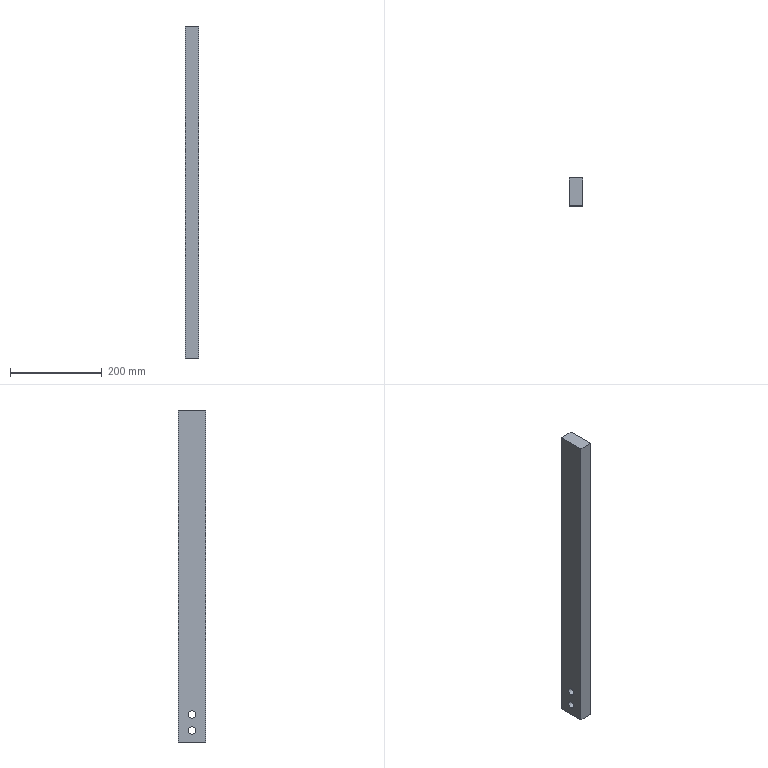Part | SolidWorks | features Cut 1, Extrusion 1, ICE 1 | 1 solid | 10 faces | box 30 x 60 x 725 mm | volume 1292936 mm3 | plane 6 | cylinder 4 | commonest cylinder face diameters 16 x4
STEP:
#1=CARTESIAN_POINT('',(15.,0.,-66.));
#2=VERTEX_POINT('',#1);
#3=CARTESIAN_POINT('',(15.,0.,-50.));
#4=VERTEX_POINT('',#3);
#5=CARTESIAN_POINT('',(15.,0.,-58.));
#6=DIRECTION('',(-1.,0.,0.));
#7=DIRECTION('',(0.,0.,1.));
#8=AXIS2_PLACEMENT_3D('',#5,#6,#7);
#9=CIRCLE('',#8,8.);
#10=EDGE_CURVE('',#2,#4,#9,.T.);
#11=ORIENTED_EDGE('',*,*,#10,.F.);
#12=CARTESIAN_POINT('',(-15.,0.,-66.));
#13=VERTEX_POINT('',#12);
#14=CARTESIAN_POINT('',(15.,0.,-66.));
#15=DIRECTION('',(-1.,0.,0.));
#16=VECTOR('',#15,1000.);
#17=LINE('',#14,#16);
#18=EDGE_CURVE('',#2,#13,#17,.T.);
#19=ORIENTED_EDGE('',*,*,#18,.T.);
#20=CARTESIAN_POINT('',(-15.,0.,-50.));
#21=VERTEX_POINT('',#20);
#22=CARTESIAN_POINT('',(-15.,0.,-58.));
#23=DIRECTION('',(-1.,0.,0.));
#24=DIRECTION('',(0.,0.,1.));
#25=AXIS2_PLACEMENT_3D('',#22,#23,#24);
#26=CIRCLE('',#25,8.);
#27=EDGE_CURVE('',#13,#21,#26,.T.);
#28=ORIENTED_EDGE('',*,*,#27,.T.);
#29=CARTESIAN_POINT('',(15.,0.,-50.));
#30=DIRECTION('',(-1.,0.,0.));
#31=VECTOR('',#30,1000.);
#32=LINE('',#29,#31);
#33=EDGE_CURVE('',#4,#21,#32,.T.);
#34=ORIENTED_EDGE('',*,*,#33,.F.);
#35=EDGE_LOOP('',(#11,#19,#28,#34));
#36=FACE_OUTER_BOUND('',#35,.T.);
#37=CARTESIAN_POINT('',(15.,0.,-58.));
#38=DIRECTION('',(-1.,0.,0.));
#39=DIRECTION('',(0.,0.,1.));
#40=AXIS2_PLACEMENT_3D('',#37,#38,#39);
#41=CYLINDRICAL_SURFACE('',#40,8.);
#42=ADVANCED_FACE('',(#36),#41,.F.);
#43=CARTESIAN_POINT('',(15.,0.,-31.));
#44=VERTEX_POINT('',#43);
#45=CARTESIAN_POINT('',(15.,0.,-15.));
#46=VERTEX_POINT('',#45);
#47=CARTESIAN_POINT('',(15.,0.,-23.));
#48=DIRECTION('',(-1.,0.,0.));
#49=DIRECTION('',(0.,0.,1.));
#50=AXIS2_PLACEMENT_3D('',#47,#48,#49);
#51=CIRCLE('',#50,8.);
#52=EDGE_CURVE('',#44,#46,#51,.T.);
#53=ORIENTED_EDGE('',*,*,#52,.F.);
#54=CARTESIAN_POINT('',(-15.,0.,-31.));
#55=VERTEX_POINT('',#54);
#56=CARTESIAN_POINT('',(15.,0.,-31.));
#57=DIRECTION('',(-1.,0.,0.));
#58=VECTOR('',#57,1000.);
#59=LINE('',#56,#58);
#60=EDGE_CURVE('',#44,#55,#59,.T.);
#61=ORIENTED_EDGE('',*,*,#60,.T.);
#62=CARTESIAN_POINT('',(-15.,0.,-15.));
#63=VERTEX_POINT('',#62);
#64=CARTESIAN_POINT('',(-15.,0.,-23.));
#65=DIRECTION('',(-1.,0.,0.));
#66=DIRECTION('',(0.,0.,1.));
#67=AXIS2_PLACEMENT_3D('',#64,#65,#66);
#68=CIRCLE('',#67,8.);
#69=EDGE_CURVE('',#55,#63,#68,.T.);
#70=ORIENTED_EDGE('',*,*,#69,.T.);
#71=CARTESIAN_POINT('',(15.,0.,-15.));
#72=DIRECTION('',(-1.,0.,0.));
#73=VECTOR('',#72,1000.);
#74=LINE('',#71,#73);
#75=EDGE_CURVE('',#46,#63,#74,.T.);
#76=ORIENTED_EDGE('',*,*,#75,.F.);
#77=EDGE_LOOP('',(#53,#61,#70,#76));
#78=FACE_OUTER_BOUND('',#77,.T.);
#79=CARTESIAN_POINT('',(15.,0.,-23.));
#80=DIRECTION('',(-1.,0.,0.));
#81=DIRECTION('',(0.,0.,1.));
#82=AXIS2_PLACEMENT_3D('',#79,#80,#81);
#83=CYLINDRICAL_SURFACE('',#82,8.);
#84=ADVANCED_FACE('',(#78),#83,.F.);
#85=CARTESIAN_POINT('',(15.,0.,-58.));
#86=DIRECTION('',(-1.,0.,0.));
#87=DIRECTION('',(0.,0.,1.));
#88=AXIS2_PLACEMENT_3D('',#85,#86,#87);
#89=CIRCLE('',#88,8.);
#90=EDGE_CURVE('',#4,#2,#89,.T.);
#91=ORIENTED_EDGE('',*,*,#90,.T.);
#92=ORIENTED_EDGE('',*,*,#10,.T.);
#93=EDGE_LOOP('',(#91,#92));
#94=FACE_BOUND('',#93,.T.);
#95=CARTESIAN_POINT('',(15.,0.,-23.));
#96=DIRECTION('',(-1.,0.,0.));
#97=DIRECTION('',(0.,0.,1.));
#98=AXIS2_PLACEMENT_3D('',#95,#96,#97);
#99=CIRCLE('',#98,8.);
#100=EDGE_CURVE('',#46,#44,#99,.T.);
#101=ORIENTED_EDGE('',*,*,#100,.T.);
#102=ORIENTED_EDGE('',*,*,#52,.T.);
#103=EDGE_LOOP('',(#101,#102));
#104=FACE_BOUND('',#103,.T.);
#105=CARTESIAN_POINT('',(15.,-30.,642.));
#106=VERTEX_POINT('',#105);
#107=CARTESIAN_POINT('',(15.,-30.,-83.));
#108=VERTEX_POINT('',#107);
#109=CARTESIAN_POINT('',(15.,-30.,642.));
#110=DIRECTION('',(0.,0.,-1.));
#111=VECTOR('',#110,1000.);
#112=LINE('',#109,#111);
#113=EDGE_CURVE('',#106,#108,#112,.T.);
#114=ORIENTED_EDGE('',*,*,#113,.T.);
#115=CARTESIAN_POINT('',(15.,30.,-83.));
#116=VERTEX_POINT('',#115);
#117=CARTESIAN_POINT('',(15.,30.,-83.));
#118=DIRECTION('',(0.,-1.,0.));
#119=VECTOR('',#118,1000.);
#120=LINE('',#117,#119);
#121=EDGE_CURVE('',#116,#108,#120,.T.);
#122=ORIENTED_EDGE('',*,*,#121,.F.);
#123=CARTESIAN_POINT('',(15.,30.,642.));
#124=VERTEX_POINT('',#123);
#125=CARTESIAN_POINT('',(15.,30.,642.));
#126=DIRECTION('',(0.,0.,-1.));
#127=VECTOR('',#126,1000.);
#128=LINE('',#125,#127);
#129=EDGE_CURVE('',#124,#116,#128,.T.);
#130=ORIENTED_EDGE('',*,*,#129,.F.);
#131=CARTESIAN_POINT('',(15.,-30.,642.));
#132=DIRECTION('',(0.,1.,0.));
#133=VECTOR('',#132,1000.);
#134=LINE('',#131,#133);
#135=EDGE_CURVE('',#106,#124,#134,.T.);
#136=ORIENTED_EDGE('',*,*,#135,.F.);
#137=EDGE_LOOP('',(#114,#122,#130,#136));
#138=FACE_OUTER_BOUND('',#137,.T.);
#139=CARTESIAN_POINT('',(15.,-30.,642.));
#140=DIRECTION('',(-1.,0.,0.));
#141=DIRECTION('',(0.,0.,1.));
#142=AXIS2_PLACEMENT_3D('',#139,#140,#141);
#143=PLANE('',#142);
#144=ADVANCED_FACE('',(#94,#104,#138),#143,.F.);
#145=ORIENTED_EDGE('',*,*,#129,.T.);
#146=CARTESIAN_POINT('',(-15.,30.,-83.));
#147=VERTEX_POINT('',#146);
#148=CARTESIAN_POINT('',(-15.,30.,-83.));
#149=DIRECTION('',(1.,0.,0.));
#150=VECTOR('',#149,1000.);
#151=LINE('',#148,#150);
#152=EDGE_CURVE('',#147,#116,#151,.T.);
#153=ORIENTED_EDGE('',*,*,#152,.F.);
#154=CARTESIAN_POINT('',(-15.,30.,642.));
#155=VERTEX_POINT('',#154);
#156=CARTESIAN_POINT('',(-15.,30.,642.));
#157=DIRECTION('',(0.,0.,-1.));
#158=VECTOR('',#157,1000.);
#159=LINE('',#156,#158);
#160=EDGE_CURVE('',#155,#147,#159,.T.);
#161=ORIENTED_EDGE('',*,*,#160,.F.);
#162=CARTESIAN_POINT('',(-15.,30.,642.));
#163=DIRECTION('',(-1.,0.,0.));
#164=VECTOR('',#163,1000.);
#165=LINE('',#162,#164);
#166=EDGE_CURVE('',#124,#155,#165,.T.);
#167=ORIENTED_EDGE('',*,*,#166,.F.);
#168=EDGE_LOOP('',(#145,#153,#161,#167));
#169=FACE_OUTER_BOUND('',#168,.T.);
#170=CARTESIAN_POINT('',(-15.,30.,642.));
#171=DIRECTION('',(0.,-1.,0.));
#172=DIRECTION('',(0.,0.,-1.));
#173=AXIS2_PLACEMENT_3D('',#170,#171,#172);
#174=PLANE('',#173);
#175=ADVANCED_FACE('',(#169),#174,.F.);
#176=CARTESIAN_POINT('',(-15.,0.,-58.));
#177=DIRECTION('',(-1.,0.,0.));
#178=DIRECTION('',(0.,0.,1.));
#179=AXIS2_PLACEMENT_3D('',#176,#177,#178);
#180=CIRCLE('',#179,8.);
#181=EDGE_CURVE('',#21,#13,#180,.T.);
#182=ORIENTED_EDGE('',*,*,#181,.F.);
#183=ORIENTED_EDGE('',*,*,#27,.F.);
#184=EDGE_LOOP('',(#182,#183));
#185=FACE_BOUND('',#184,.T.);
#186=CARTESIAN_POINT('',(-15.,0.,-23.));
#187=DIRECTION('',(-1.,0.,0.));
#188=DIRECTION('',(0.,0.,1.));
#189=AXIS2_PLACEMENT_3D('',#186,#187,#188);
#190=CIRCLE('',#189,8.);
#191=EDGE_CURVE('',#63,#55,#190,.T.);
#192=ORIENTED_EDGE('',*,*,#191,.F.);
#193=ORIENTED_EDGE('',*,*,#69,.F.);
#194=EDGE_LOOP('',(#192,#193));
#195=FACE_BOUND('',#194,.T.);
#196=ORIENTED_EDGE('',*,*,#160,.T.);
#197=CARTESIAN_POINT('',(-15.,-30.,-83.));
#198=VERTEX_POINT('',#197);
#199=CARTESIAN_POINT('',(-15.,-30.,-83.));
#200=DIRECTION('',(0.,1.,0.));
#201=VECTOR('',#200,1000.);
#202=LINE('',#199,#201);
#203=EDGE_CURVE('',#198,#147,#202,.T.);
#204=ORIENTED_EDGE('',*,*,#203,.F.);
#205=CARTESIAN_POINT('',(-15.,-30.,642.));
#206=VERTEX_POINT('',#205);
#207=CARTESIAN_POINT('',(-15.,-30.,642.));
#208=DIRECTION('',(0.,0.,-1.));
#209=VECTOR('',#208,1000.);
#210=LINE('',#207,#209);
#211=EDGE_CURVE('',#206,#198,#210,.T.);
#212=ORIENTED_EDGE('',*,*,#211,.F.);
#213=CARTESIAN_POINT('',(-15.,-30.,642.));
#214=DIRECTION('',(0.,-1.,0.));
#215=VECTOR('',#214,1000.);
#216=LINE('',#213,#215);
#217=EDGE_CURVE('',#155,#206,#216,.T.);
#218=ORIENTED_EDGE('',*,*,#217,.F.);
#219=EDGE_LOOP('',(#196,#204,#212,#218));
#220=FACE_OUTER_BOUND('',#219,.T.);
#221=CARTESIAN_POINT('',(-15.,-30.,642.));
#222=DIRECTION('',(1.,0.,0.));
#223=DIRECTION('',(0.,0.,-1.));
#224=AXIS2_PLACEMENT_3D('',#221,#222,#223);
#225=PLANE('',#224);
#226=ADVANCED_FACE('',(#185,#195,#220),#225,.F.);
#227=ORIENTED_EDGE('',*,*,#211,.T.);
#228=CARTESIAN_POINT('',(15.,-30.,-83.));
#229=DIRECTION('',(-1.,0.,0.));
#230=VECTOR('',#229,1000.);
#231=LINE('',#228,#230);
#232=EDGE_CURVE('',#108,#198,#231,.T.);
#233=ORIENTED_EDGE('',*,*,#232,.F.);
#234=ORIENTED_EDGE('',*,*,#113,.F.);
#235=CARTESIAN_POINT('',(-15.,-30.,642.));
#236=DIRECTION('',(1.,0.,0.));
#237=VECTOR('',#236,1000.);
#238=LINE('',#235,#237);
#239=EDGE_CURVE('',#206,#106,#238,.T.);
#240=ORIENTED_EDGE('',*,*,#239,.F.);
#241=EDGE_LOOP('',(#227,#233,#234,#240));
#242=FACE_OUTER_BOUND('',#241,.T.);
#243=CARTESIAN_POINT('',(-15.,-30.,642.));
#244=DIRECTION('',(0.,1.,0.));
#245=DIRECTION('',(0.,0.,1.));
#246=AXIS2_PLACEMENT_3D('',#243,#244,#245);
#247=PLANE('',#246);
#248=ADVANCED_FACE('',(#242),#247,.F.);
#249=ORIENTED_EDGE('',*,*,#135,.T.);
#250=ORIENTED_EDGE('',*,*,#166,.T.);
#251=ORIENTED_EDGE('',*,*,#217,.T.);
#252=ORIENTED_EDGE('',*,*,#239,.T.);
#253=EDGE_LOOP('',(#249,#250,#251,#252));
#254=FACE_OUTER_BOUND('',#253,.T.);
#255=CARTESIAN_POINT('',(0.,0.,642.));
#256=DIRECTION('',(0.,0.,-1.));
#257=DIRECTION('',(-1.,0.,0.));
#258=AXIS2_PLACEMENT_3D('',#255,#256,#257);
#259=PLANE('',#258);
#260=ADVANCED_FACE('',(#254),#259,.F.);
#261=ORIENTED_EDGE('',*,*,#152,.T.);
#262=ORIENTED_EDGE('',*,*,#121,.T.);
#263=ORIENTED_EDGE('',*,*,#232,.T.);
#264=ORIENTED_EDGE('',*,*,#203,.T.);
#265=EDGE_LOOP('',(#261,#262,#263,#264));
#266=FACE_OUTER_BOUND('',#265,.T.);
#267=CARTESIAN_POINT('',(0.,0.,-83.));
#268=DIRECTION('',(0.,0.,-1.));
#269=DIRECTION('',(-1.,0.,0.));
#270=AXIS2_PLACEMENT_3D('',#267,#268,#269);
#271=PLANE('',#270);
#272=ADVANCED_FACE('',(#266),#271,.T.);
#273=ORIENTED_EDGE('',*,*,#60,.F.);
#274=ORIENTED_EDGE('',*,*,#100,.F.);
#275=ORIENTED_EDGE('',*,*,#75,.T.);
#276=ORIENTED_EDGE('',*,*,#191,.T.);
#277=EDGE_LOOP('',(#273,#274,#275,#276));
#278=FACE_OUTER_BOUND('',#277,.T.);
#279=CARTESIAN_POINT('',(15.,0.,-23.));
#280=DIRECTION('',(-1.,0.,0.));
#281=DIRECTION('',(0.,0.,1.));
#282=AXIS2_PLACEMENT_3D('',#279,#280,#281);
#283=CYLINDRICAL_SURFACE('',#282,8.);
#284=ADVANCED_FACE('',(#278),#283,.F.);
#285=ORIENTED_EDGE('',*,*,#18,.F.);
#286=ORIENTED_EDGE('',*,*,#90,.F.);
#287=ORIENTED_EDGE('',*,*,#33,.T.);
#288=ORIENTED_EDGE('',*,*,#181,.T.);
#289=EDGE_LOOP('',(#285,#286,#287,#288));
#290=FACE_OUTER_BOUND('',#289,.T.);
#291=CARTESIAN_POINT('',(15.,0.,-58.));
#292=DIRECTION('',(-1.,0.,0.));
#293=DIRECTION('',(0.,0.,1.));
#294=AXIS2_PLACEMENT_3D('',#291,#292,#293);
#295=CYLINDRICAL_SURFACE('',#294,8.);
#296=ADVANCED_FACE('',(#290),#295,.F.);
#297=CLOSED_SHELL('',(#42,#84,#144,#175,#226,#248,#260,#272,#284,#296));
#298=MANIFOLD_SOLID_BREP('',#297);
#299=CARTESIAN_POINT('',(0.,0.,0.));
#300=DIRECTION('',(0.,0.,1.));
#301=DIRECTION('',(1.,0.,0.));
#302=AXIS2_PLACEMENT_3D('',#299,#300,#301);
#303=(LENGTH_UNIT()NAMED_UNIT(*)SI_UNIT(.MILLI.,.METRE.));
#304=UNCERTAINTY_MEASURE_WITH_UNIT(LENGTH_MEASURE(0.00001),#303,'','');
#305=(NAMED_UNIT(*)PLANE_ANGLE_UNIT()SI_UNIT($,.RADIAN.));
#306=(NAMED_UNIT(*)SI_UNIT($,.STERADIAN.)SOLID_ANGLE_UNIT());
#307=(GEOMETRIC_REPRESENTATION_CONTEXT(3)GLOBAL_UNCERTAINTY_ASSIGNED_CONTEXT((#304))GLOBAL_UNIT_ASSIGNED_CONTEXT((#303,#305,#306))REPRESENTATION_CONTEXT('',''));
#308=ADVANCED_BREP_SHAPE_REPRESENTATION('',(#298,#302),#307);